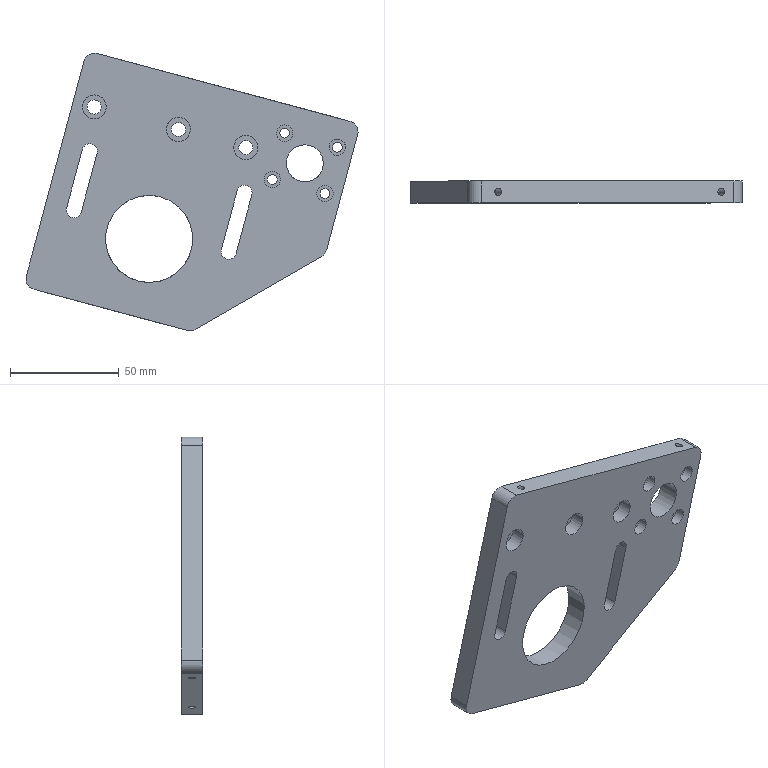CAM job | NX | 3+2 milling, drilling | part box 152.311 x 10 x 127.359 mm | stock box 160.682 x 12 x 147.954 mm
Tools:
number,name,description,diameter,corner_radius,flute_length,length,flutes
4,D4,平底铣刀-粗,4.0,0.0,25.0,75.0,2
6,D6,平底铣刀-粗,6.0,0.0,25.0,75.0,2
9,D10,平底铣刀-粗,10.0,0.0,35.0,75.0,2
7,D6-J,平底铣刀-精,6.0,0.0,25.0,75.0,2
10,D10-J,平底铣刀-精,10.0,0.0,35.0,75.0,2
1,D80R0.8飞刀,圆鼻刀-粗,80.0,0.8,50.0,75.0,2
1,D80R0.8飞刀-J,圆鼻刀-精,80.0,0.8,50.0,75.0,2
2,D6倒角刀,倒角刀,6.0,0.0,3.0,25.0,2
11,ZT4.5,钻头,4.5,0.0,35.0,50.0,2
17,ZT6.5,钻头,6.5,0.0,35.0,50.0,2
Operations:
program,operation,operation_type,tool,method,geometry_group,spindle_rpm,surface_speed,feed_per_tooth,feed_cut,feed_plunge,cut_length_mm,path_length_mm,cut_time_min,machine_time_min
B,底壁铣飞面开粗_COPY,VolumeBased25DMillingOperation,D80R0.8飞刀,分层开粗-切深K-步距G,W-B,2800.0,703.696,0.5357,3000.0,100.0,1977.224,2189.107,0.6591,0.6803
B,底壁铣飞面精光_COPY,VolumeBased25DMillingOperation,D80R0.8飞刀-J,侧刃精光-切深K-步距G,W-B,4000.0,1005.28,0.125,1000.0,100.0,493.754,529.754,0.4938,0.4974
B,钻倒角_1,Operation,D6倒角刀,METHOD,W-B,8000.0,150.796,0.0625,1000.0,0.0,22.2,162.987,0.0222,0.0363
B,平面去毛刺6X45L_COPY,SurfaceContour,D6倒角刀,爬面_倒角-切深0-步距G,W-B,6500.0,122.519,0.1154,1500.0,100.0,890.365,1530.732,0.5936,0.6576
A,顶面,FaceMilling,D80R0.8飞刀,侧刃精光-切深K-步距G,W-A,4000.0,1005.31,0.125,1000.0,100.0,740.0,776.0,0.74,0.7436
A,型腔铣开粗-中_COPY,CavityMilling,D10,分层开粗-切深K-步距G,W-A,8000.0,251.32,0.25,4000.0,100.0,32639.498,33764.347,8.16,8.325
A,打点0.8,Operation,D6倒角刀,METHOD,W-A,8000.0,150.796,0.0312,500.0,0.0,1.8,43.6,0.0036,0.0078
A,沉头孔打点-深0.8,Operation,D6倒角刀,NONE,W-A,8000.0,150.796,0.0312,500.0,90.0,14.4,244.268,0.0288,0.0518
A,沉头孔-钻孔0段,Operation,ZT4.5,NONE,W-A,2800.0,39.584,0.0179,100.0,90.0,57.408,226.881,0.5741,0.591
A,沉头孔-钻孔0段_2,Operation,ZT6.5,NONE,W-A,1200.0,24.504,0.0625,150.0,90.0,44.858,203.745,0.2991,0.3149
A,通孔-12.5-25,Operation,ZT6.5,NONE,W-A,800.0,30.159,0.125,200.0,90.0,14.953,69.906,0.0748,0.0803
A,通腰槽粗_1,VolumeBased25DMillingOperation,D6,METHOD,W-A,6000.0,113.0,0.2083,2500.0,100.0,6439.383,6610.124,2.576,2.593
A,铣孔开粗D8_1,CylinderMilling,D10,NONE,W-A,8000.0,201.062,0.075,1200.0,100.0,502.155,552.155,0.4185,0.4235
A,铣孔开粗D6_1,CylinderMilling,D6,NONE,W-A,8000.0,150.796,0.075,1200.0,100.0,701.552,911.552,0.5846,0.6056
A,铣孔开粗D4_1,CylinderMilling,D4,NONE,W-A,8000.0,100.531,0.075,1200.0,100.0,753.643,998.643,0.628,0.6525
A,铣孔精光D4_1,CylinderMilling,D4,精光步距切深关,W-A,8000.0,100.531,0.0312,500.0,100.0,114.03,359.03,0.2281,0.2526
A,铣孔精光D6_1,CylinderMilling,D6-J,精光步距切深关,W-A,8000.0,150.796,0.0312,500.0,100.0,134.835,346.335,0.2697,0.2908
A,腰槽精_1,VolumeBased25DMillingOperation,D6-J,METHOD,W-A,6000.0,113.0,0.0667,600.0,100.0,245.476,461.42,0.4091,0.4307
A,仅选体,SurfaceContour,D6倒角刀,METHOD,W-A,8000.0,150.796,0.1875,3000.0,100.0,812.761,1155.498,0.2709,0.3052
A,铣倒角_1,PlanarMilling,D6倒角刀,NONE,W-A,8000.0,150.796,0.0312,500.0,100.0,134.615,346.029,0.2692,0.2904
A,铣倒角_2,PlanarMilling,D6倒角刀,NONE,W-A,8000.0,150.796,0.05,800.0,100.0,133.948,328.059,0.1674,0.1868
A,铣倒角_3,PlanarMilling,D6倒角刀,METHOD,W-A,8000.0,150.796,0.0625,1000.0,100.0,57.549,99.549,0.0575,0.0617
A,铣倒角_4,PlanarMilling,D6倒角刀,METHOD,W-A,8000.0,150.796,0.05,800.0,100.0,132.947,173.947,0.1662,0.1703
A,底壁铣精光侧面-中_COPY,VolumeBased25DMillingOperation,D6-J,侧刃精光-切深K-步距G,W-A,8000.0,150.792,0.0625,1000.0,100.0,41.363,78.763,0.0414,0.0451
A,底壁铣精光侧面-中_COPY_COPY,VolumeBased25DMillingOperation,D6-J,侧刃精光-切深K-步距G,W-A,8000.0,150.792,0.0625,1000.0,100.0,113.492,150.592,0.1135,0.1172
A,外形半精_2,VolumeBased25DMillingOperation,D10-J,METHOD,W-A,8000.0,251.327,0.0625,1000.0,100.0,484.163,543.362,0.4842,0.4901